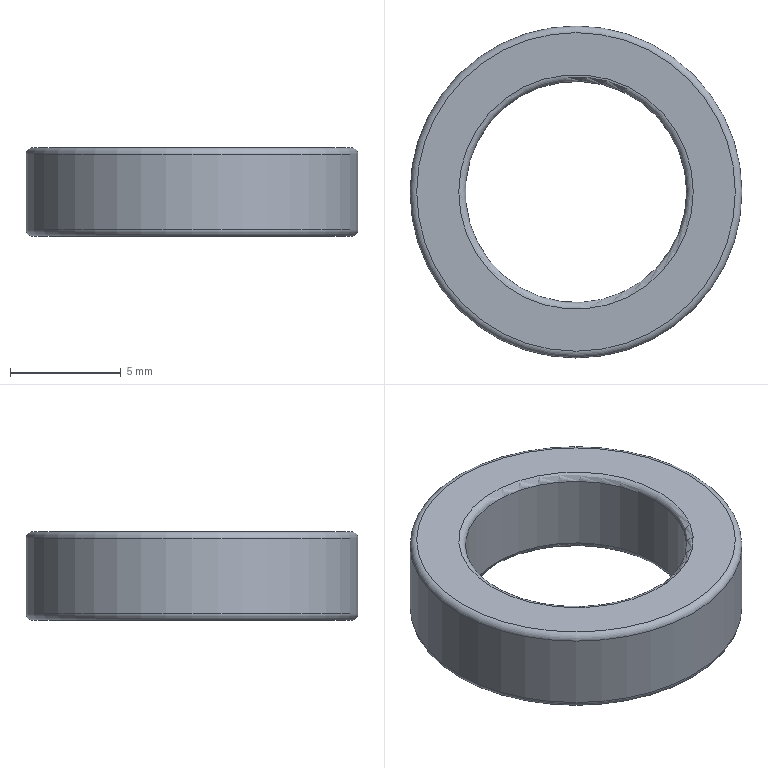Part | NX | 1 solid | 8 faces | box 15 x 15 x 4 mm | volume 389.665 mm3 | torus 4 | plane 2 | cylinder 2 | commonest cylinder face diameters 10 x1 15 x1
STEP:
#1=CARTESIAN_POINT('',(5.3,0.,4.));
#2=VERTEX_POINT('',#1);
#3=CARTESIAN_POINT('',(0.,0.,4.));
#4=DIRECTION('',(0.,0.,1.));
#5=DIRECTION('',(1.,0.,0.));
#6=AXIS2_PLACEMENT_3D('',#3,#4,#5);
#7=CIRCLE('',#6,5.3);
#8=EDGE_CURVE('',#2,#2,#7,.F.);
#9=ORIENTED_EDGE('',*,*,#8,.T.);
#10=EDGE_LOOP('',(#9));
#11=FACE_BOUND('',#10,.T.);
#12=CARTESIAN_POINT('',(7.2,0.,4.));
#13=VERTEX_POINT('',#12);
#14=CARTESIAN_POINT('',(0.,0.,4.));
#15=DIRECTION('',(0.,0.,1.));
#16=DIRECTION('',(1.,0.,0.));
#17=AXIS2_PLACEMENT_3D('',#14,#15,#16);
#18=CIRCLE('',#17,7.2);
#19=EDGE_CURVE('',#13,#13,#18,.T.);
#20=ORIENTED_EDGE('',*,*,#19,.T.);
#21=EDGE_LOOP('',(#20));
#22=FACE_BOUND('',#21,.T.);
#23=CARTESIAN_POINT('',(0.,0.,4.));
#24=DIRECTION('',(0.,0.,1.));
#25=DIRECTION('',(1.,0.,0.));
#26=AXIS2_PLACEMENT_3D('',#23,#24,#25);
#27=PLANE('',#26);
#28=ADVANCED_FACE('',(#11,#22),#27,.T.);
#29=CARTESIAN_POINT('',(5.3,0.,0.));
#30=VERTEX_POINT('',#29);
#31=CARTESIAN_POINT('',(0.,0.,0.));
#32=DIRECTION('',(0.,0.,1.));
#33=DIRECTION('',(1.,0.,0.));
#34=AXIS2_PLACEMENT_3D('',#31,#32,#33);
#35=CIRCLE('',#34,5.3);
#36=EDGE_CURVE('',#30,#30,#35,.T.);
#37=ORIENTED_EDGE('',*,*,#36,.T.);
#38=EDGE_LOOP('',(#37));
#39=FACE_BOUND('',#38,.T.);
#40=CARTESIAN_POINT('',(7.2,0.,0.));
#41=VERTEX_POINT('',#40);
#42=CARTESIAN_POINT('',(0.,0.,0.));
#43=DIRECTION('',(0.,0.,1.));
#44=DIRECTION('',(1.,0.,0.));
#45=AXIS2_PLACEMENT_3D('',#42,#43,#44);
#46=CIRCLE('',#45,7.2);
#47=EDGE_CURVE('',#41,#41,#46,.F.);
#48=ORIENTED_EDGE('',*,*,#47,.T.);
#49=EDGE_LOOP('',(#48));
#50=FACE_BOUND('',#49,.T.);
#51=CARTESIAN_POINT('',(0.,0.,0.));
#52=DIRECTION('',(0.,0.,1.));
#53=DIRECTION('',(1.,0.,0.));
#54=AXIS2_PLACEMENT_3D('',#51,#52,#53);
#55=PLANE('',#54);
#56=ADVANCED_FACE('',(#39,#50),#55,.F.);
#57=CARTESIAN_POINT('',(7.5,0.,0.3));
#58=VERTEX_POINT('',#57);
#59=CARTESIAN_POINT('',(0.,0.,0.3));
#60=DIRECTION('',(0.,0.,1.));
#61=DIRECTION('',(1.,0.,0.));
#62=AXIS2_PLACEMENT_3D('',#59,#60,#61);
#63=CIRCLE('',#62,7.5);
#64=EDGE_CURVE('',#58,#58,#63,.T.);
#65=ORIENTED_EDGE('',*,*,#64,.T.);
#66=EDGE_LOOP('',(#65));
#67=FACE_BOUND('',#66,.T.);
#68=CARTESIAN_POINT('',(7.5,0.,3.7));
#69=VERTEX_POINT('',#68);
#70=CARTESIAN_POINT('',(0.,0.,3.7));
#71=DIRECTION('',(0.,0.,1.));
#72=DIRECTION('',(1.,0.,0.));
#73=AXIS2_PLACEMENT_3D('',#70,#71,#72);
#74=CIRCLE('',#73,7.5);
#75=EDGE_CURVE('',#69,#69,#74,.F.);
#76=ORIENTED_EDGE('',*,*,#75,.T.);
#77=EDGE_LOOP('',(#76));
#78=FACE_BOUND('',#77,.T.);
#79=CARTESIAN_POINT('',(0.,0.,4.));
#80=DIRECTION('',(0.,0.,-1.));
#81=DIRECTION('',(-1.,0.,0.));
#82=AXIS2_PLACEMENT_3D('',#79,#80,#81);
#83=CYLINDRICAL_SURFACE('',#82,7.5);
#84=ADVANCED_FACE('',(#67,#78),#83,.T.);
#85=CARTESIAN_POINT('',(5.,0.,0.3));
#86=VERTEX_POINT('',#85);
#87=CARTESIAN_POINT('',(0.,0.,0.3));
#88=DIRECTION('',(0.,0.,1.));
#89=DIRECTION('',(1.,0.,0.));
#90=AXIS2_PLACEMENT_3D('',#87,#88,#89);
#91=CIRCLE('',#90,5.);
#92=EDGE_CURVE('',#86,#86,#91,.F.);
#93=ORIENTED_EDGE('',*,*,#92,.T.);
#94=EDGE_LOOP('',(#93));
#95=FACE_BOUND('',#94,.T.);
#96=CARTESIAN_POINT('',(5.,0.,3.7));
#97=VERTEX_POINT('',#96);
#98=CARTESIAN_POINT('',(0.,0.,3.7));
#99=DIRECTION('',(0.,0.,1.));
#100=DIRECTION('',(1.,0.,0.));
#101=AXIS2_PLACEMENT_3D('',#98,#99,#100);
#102=CIRCLE('',#101,5.);
#103=EDGE_CURVE('',#97,#97,#102,.T.);
#104=ORIENTED_EDGE('',*,*,#103,.T.);
#105=EDGE_LOOP('',(#104));
#106=FACE_BOUND('',#105,.T.);
#107=CARTESIAN_POINT('',(0.,0.,4.));
#108=DIRECTION('',(0.,0.,-1.));
#109=DIRECTION('',(-1.,0.,0.));
#110=AXIS2_PLACEMENT_3D('',#107,#108,#109);
#111=CYLINDRICAL_SURFACE('',#110,5.);
#112=ADVANCED_FACE('',(#95,#106),#111,.F.);
#113=ORIENTED_EDGE('',*,*,#92,.F.);
#114=EDGE_LOOP('',(#113));
#115=FACE_BOUND('',#114,.T.);
#116=ORIENTED_EDGE('',*,*,#36,.F.);
#117=EDGE_LOOP('',(#116));
#118=FACE_BOUND('',#117,.T.);
#119=CARTESIAN_POINT('',(0.,0.,0.3));
#120=DIRECTION('',(0.,0.,1.));
#121=DIRECTION('',(1.,0.,0.));
#122=AXIS2_PLACEMENT_3D('',#119,#120,#121);
#123=TOROIDAL_SURFACE('',#122,5.3,0.3);
#124=ADVANCED_FACE('',(#115,#118),#123,.T.);
#125=ORIENTED_EDGE('',*,*,#8,.F.);
#126=EDGE_LOOP('',(#125));
#127=FACE_BOUND('',#126,.T.);
#128=ORIENTED_EDGE('',*,*,#103,.F.);
#129=EDGE_LOOP('',(#128));
#130=FACE_BOUND('',#129,.T.);
#131=CARTESIAN_POINT('',(0.,0.,3.7));
#132=DIRECTION('',(0.,0.,1.));
#133=DIRECTION('',(1.,0.,0.));
#134=AXIS2_PLACEMENT_3D('',#131,#132,#133);
#135=TOROIDAL_SURFACE('',#134,5.3,0.3);
#136=ADVANCED_FACE('',(#127,#130),#135,.T.);
#137=ORIENTED_EDGE('',*,*,#47,.F.);
#138=EDGE_LOOP('',(#137));
#139=FACE_BOUND('',#138,.T.);
#140=ORIENTED_EDGE('',*,*,#64,.F.);
#141=EDGE_LOOP('',(#140));
#142=FACE_BOUND('',#141,.T.);
#143=CARTESIAN_POINT('',(0.,0.,0.3));
#144=DIRECTION('',(0.,0.,1.));
#145=DIRECTION('',(1.,0.,0.));
#146=AXIS2_PLACEMENT_3D('',#143,#144,#145);
#147=TOROIDAL_SURFACE('',#146,7.2,0.3);
#148=ADVANCED_FACE('',(#139,#142),#147,.T.);
#149=ORIENTED_EDGE('',*,*,#75,.F.);
#150=EDGE_LOOP('',(#149));
#151=FACE_BOUND('',#150,.T.);
#152=ORIENTED_EDGE('',*,*,#19,.F.);
#153=EDGE_LOOP('',(#152));
#154=FACE_BOUND('',#153,.T.);
#155=CARTESIAN_POINT('',(0.,0.,3.7));
#156=DIRECTION('',(0.,0.,1.));
#157=DIRECTION('',(1.,0.,0.));
#158=AXIS2_PLACEMENT_3D('',#155,#156,#157);
#159=TOROIDAL_SURFACE('',#158,7.2,0.3);
#160=ADVANCED_FACE('',(#151,#154),#159,.T.);
#161=CLOSED_SHELL('',(#28,#56,#84,#112,#124,#136,#148,#160));
#162=MANIFOLD_SOLID_BREP('',#161);
#163=(LENGTH_UNIT()NAMED_UNIT(*)SI_UNIT(.MILLI.,.METRE.));
#164=UNCERTAINTY_MEASURE_WITH_UNIT(LENGTH_MEASURE(0.00001),#163,'','');
#165=(NAMED_UNIT(*)PLANE_ANGLE_UNIT()SI_UNIT($,.RADIAN.));
#166=(NAMED_UNIT(*)SI_UNIT($,.STERADIAN.)SOLID_ANGLE_UNIT());
#167=(GEOMETRIC_REPRESENTATION_CONTEXT(3)GLOBAL_UNCERTAINTY_ASSIGNED_CONTEXT((#164))GLOBAL_UNIT_ASSIGNED_CONTEXT((#163,#165,#166))REPRESENTATION_CONTEXT('',''));
#168=ADVANCED_BREP_SHAPE_REPRESENTATION('',(#162),#167);